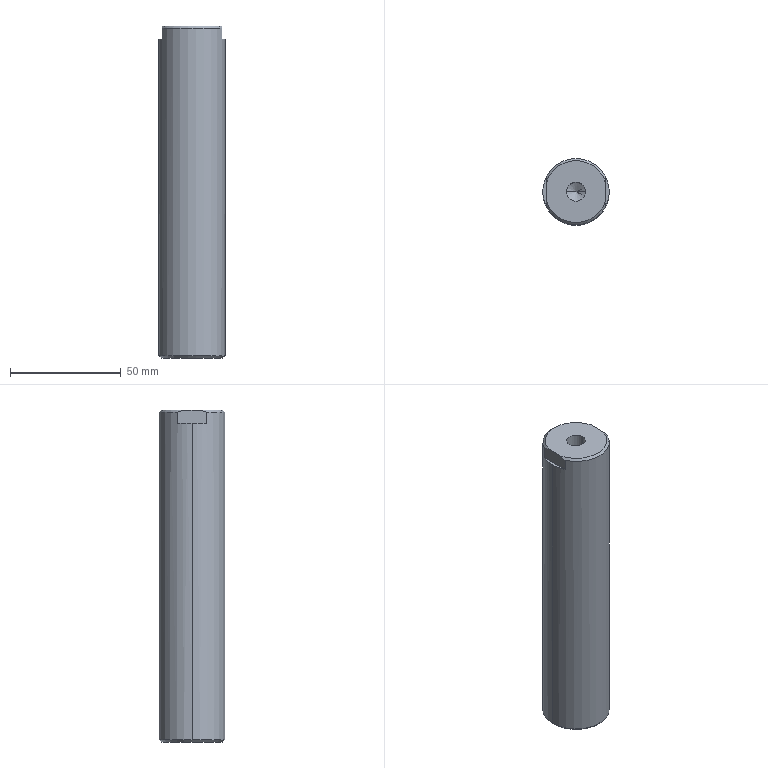Part | SolidWorks | features BaseBody 1 | 1 solid | 20 faces | box 30 x 30 x 150 mm | volume 102856 mm3 | cone 8 | cylinder 6 | plane 6 | commonest cylinder face diameters 8.5 x4 30 x2
STEP:
#1=CARTESIAN_POINT('',(-4.25,0.,125.));
#2=VERTEX_POINT('',#1);
#3=CARTESIAN_POINT('',(4.25,0.,125.));
#4=VERTEX_POINT('',#3);
#5=CARTESIAN_POINT('',(0.,0.,125.));
#6=DIRECTION('',(0.,0.,1.));
#7=DIRECTION('',(1.,0.,0.));
#8=AXIS2_PLACEMENT_3D('',#5,#6,#7);
#9=CIRCLE('',#8,4.25);
#10=EDGE_CURVE('',#2,#4,#9,.T.);
#11=ORIENTED_EDGE('',*,*,#10,.F.);
#12=CARTESIAN_POINT('',(-4.25,0.,150.));
#13=VERTEX_POINT('',#12);
#14=CARTESIAN_POINT('',(-4.25,0.,150.));
#15=DIRECTION('',(0.,0.,1.));
#16=VECTOR('',#15,1000.);
#17=LINE('',#14,#16);
#18=EDGE_CURVE('',#2,#13,#17,.T.);
#19=ORIENTED_EDGE('',*,*,#18,.T.);
#20=CARTESIAN_POINT('',(4.25,0.,150.));
#21=VERTEX_POINT('',#20);
#22=CARTESIAN_POINT('',(0.,0.,150.));
#23=DIRECTION('',(0.,0.,1.));
#24=DIRECTION('',(1.,0.,0.));
#25=AXIS2_PLACEMENT_3D('',#22,#23,#24);
#26=CIRCLE('',#25,4.25);
#27=EDGE_CURVE('',#13,#21,#26,.T.);
#28=ORIENTED_EDGE('',*,*,#27,.T.);
#29=CARTESIAN_POINT('',(4.25,0.,150.));
#30=DIRECTION('',(0.,0.,1.));
#31=VECTOR('',#30,1000.);
#32=LINE('',#29,#31);
#33=EDGE_CURVE('',#4,#21,#32,.T.);
#34=ORIENTED_EDGE('',*,*,#33,.F.);
#35=EDGE_LOOP('',(#11,#19,#28,#34));
#36=FACE_OUTER_BOUND('',#35,.T.);
#37=CARTESIAN_POINT('',(0.,0.,150.));
#38=DIRECTION('',(0.,0.,1.));
#39=DIRECTION('',(1.,0.,0.));
#40=AXIS2_PLACEMENT_3D('',#37,#38,#39);
#41=CYLINDRICAL_SURFACE('',#40,4.25);
#42=ADVANCED_FACE('',(#36),#41,.F.);
#43=CARTESIAN_POINT('',(0.,0.,122.446));
#44=VERTEX_POINT('',#43);
#45=CARTESIAN_POINT('',(4.25,0.,125.));
#46=DIRECTION('',(0.8572,0.,0.515));
#47=VECTOR('',#46,1000.);
#48=LINE('',#45,#47);
#49=EDGE_CURVE('',#44,#4,#48,.T.);
#50=ORIENTED_EDGE('',*,*,#49,.F.);
#51=CARTESIAN_POINT('',(-4.25,0.,125.));
#52=DIRECTION('',(-0.8572,0.,0.515));
#53=VECTOR('',#52,1000.);
#54=LINE('',#51,#53);
#55=EDGE_CURVE('',#44,#2,#54,.T.);
#56=ORIENTED_EDGE('',*,*,#55,.T.);
#57=ORIENTED_EDGE('',*,*,#10,.T.);
#58=EDGE_LOOP('',(#50,#56,#57));
#59=FACE_OUTER_BOUND('',#58,.T.);
#60=CARTESIAN_POINT('',(0.,0.,125.));
#61=DIRECTION('',(0.,0.,1.));
#62=DIRECTION('',(1.,0.,0.));
#63=AXIS2_PLACEMENT_3D('',#60,#61,#62);
#64=CONICAL_SURFACE('',#63,4.25,1.03);
#65=ADVANCED_FACE('',(#59),#64,.F.);
#66=CARTESIAN_POINT('',(4.25,0.,25.));
#67=VERTEX_POINT('',#66);
#68=CARTESIAN_POINT('',(-4.25,0.,25.));
#69=VERTEX_POINT('',#68);
#70=CARTESIAN_POINT('',(0.,0.,25.));
#71=DIRECTION('',(0.,0.,-1.));
#72=DIRECTION('',(-1.,0.,0.));
#73=AXIS2_PLACEMENT_3D('',#70,#71,#72);
#74=CIRCLE('',#73,4.25);
#75=EDGE_CURVE('',#67,#69,#74,.T.);
#76=ORIENTED_EDGE('',*,*,#75,.F.);
#77=CARTESIAN_POINT('',(4.25,0.,0.));
#78=VERTEX_POINT('',#77);
#79=CARTESIAN_POINT('',(4.25,0.,0.));
#80=DIRECTION('',(0.,0.,-1.));
#81=VECTOR('',#80,1000.);
#82=LINE('',#79,#81);
#83=EDGE_CURVE('',#67,#78,#82,.T.);
#84=ORIENTED_EDGE('',*,*,#83,.T.);
#85=CARTESIAN_POINT('',(-4.25,0.,0.));
#86=VERTEX_POINT('',#85);
#87=CARTESIAN_POINT('',(0.,0.,0.));
#88=DIRECTION('',(0.,0.,-1.));
#89=DIRECTION('',(-1.,0.,0.));
#90=AXIS2_PLACEMENT_3D('',#87,#88,#89);
#91=CIRCLE('',#90,4.25);
#92=EDGE_CURVE('',#78,#86,#91,.T.);
#93=ORIENTED_EDGE('',*,*,#92,.T.);
#94=CARTESIAN_POINT('',(-4.25,0.,0.));
#95=DIRECTION('',(0.,0.,-1.));
#96=VECTOR('',#95,1000.);
#97=LINE('',#94,#96);
#98=EDGE_CURVE('',#69,#86,#97,.T.);
#99=ORIENTED_EDGE('',*,*,#98,.F.);
#100=EDGE_LOOP('',(#76,#84,#93,#99));
#101=FACE_OUTER_BOUND('',#100,.T.);
#102=CARTESIAN_POINT('',(0.,0.,0.));
#103=DIRECTION('',(0.,0.,-1.));
#104=DIRECTION('',(-1.,0.,0.));
#105=AXIS2_PLACEMENT_3D('',#102,#103,#104);
#106=CYLINDRICAL_SURFACE('',#105,4.25);
#107=ADVANCED_FACE('',(#101),#106,.F.);
#108=CARTESIAN_POINT('',(0.,0.,27.554));
#109=VERTEX_POINT('',#108);
#110=CARTESIAN_POINT('',(-4.25,0.,25.));
#111=DIRECTION('',(-0.8572,0.,-0.515));
#112=VECTOR('',#111,1000.);
#113=LINE('',#110,#112);
#114=EDGE_CURVE('',#109,#69,#113,.T.);
#115=ORIENTED_EDGE('',*,*,#114,.F.);
#116=CARTESIAN_POINT('',(4.25,0.,25.));
#117=DIRECTION('',(0.8572,0.,-0.515));
#118=VECTOR('',#117,1000.);
#119=LINE('',#116,#118);
#120=EDGE_CURVE('',#109,#67,#119,.T.);
#121=ORIENTED_EDGE('',*,*,#120,.T.);
#122=ORIENTED_EDGE('',*,*,#75,.T.);
#123=EDGE_LOOP('',(#115,#121,#122));
#124=FACE_OUTER_BOUND('',#123,.T.);
#125=CARTESIAN_POINT('',(0.,0.,25.));
#126=DIRECTION('',(0.,0.,-1.));
#127=DIRECTION('',(-1.,0.,0.));
#128=AXIS2_PLACEMENT_3D('',#125,#126,#127);
#129=CONICAL_SURFACE('',#128,4.25,1.03);
#130=ADVANCED_FACE('',(#124),#129,.F.);
#131=CARTESIAN_POINT('',(-14.,0.,0.));
#132=VERTEX_POINT('',#131);
#133=CARTESIAN_POINT('',(14.,0.,0.));
#134=VERTEX_POINT('',#133);
#135=CARTESIAN_POINT('',(0.,0.,0.));
#136=DIRECTION('',(0.,0.,-1.));
#137=DIRECTION('',(1.,0.,0.));
#138=AXIS2_PLACEMENT_3D('',#135,#136,#137);
#139=CIRCLE('',#138,14.);
#140=EDGE_CURVE('',#132,#134,#139,.T.);
#141=ORIENTED_EDGE('',*,*,#140,.F.);
#142=CARTESIAN_POINT('',(-15.,0.,1.));
#143=VERTEX_POINT('',#142);
#144=CARTESIAN_POINT('',(-15.,0.,1.));
#145=DIRECTION('',(-0.7071,0.,0.7071));
#146=VECTOR('',#145,1000.);
#147=LINE('',#144,#146);
#148=EDGE_CURVE('',#132,#143,#147,.T.);
#149=ORIENTED_EDGE('',*,*,#148,.T.);
#150=CARTESIAN_POINT('',(15.,0.,1.));
#151=VERTEX_POINT('',#150);
#152=CARTESIAN_POINT('',(0.,0.,1.));
#153=DIRECTION('',(0.,0.,1.));
#154=DIRECTION('',(1.,0.,0.));
#155=AXIS2_PLACEMENT_3D('',#152,#153,#154);
#156=CIRCLE('',#155,15.);
#157=EDGE_CURVE('',#151,#143,#156,.T.);
#158=ORIENTED_EDGE('',*,*,#157,.F.);
#159=CARTESIAN_POINT('',(15.,0.,1.));
#160=DIRECTION('',(0.7071,0.,0.7071));
#161=VECTOR('',#160,1000.);
#162=LINE('',#159,#161);
#163=EDGE_CURVE('',#134,#151,#162,.T.);
#164=ORIENTED_EDGE('',*,*,#163,.F.);
#165=EDGE_LOOP('',(#141,#149,#158,#164));
#166=FACE_OUTER_BOUND('',#165,.T.);
#167=CARTESIAN_POINT('',(0.,0.,1.));
#168=DIRECTION('',(0.,0.,1.));
#169=DIRECTION('',(1.,0.,0.));
#170=AXIS2_PLACEMENT_3D('',#167,#168,#169);
#171=CONICAL_SURFACE('',#170,15.,0.7854);
#172=ADVANCED_FACE('',(#166),#171,.T.);
#173=CARTESIAN_POINT('',(15.,0.,144.));
#174=VERTEX_POINT('',#173);
#175=CARTESIAN_POINT('',(13.5,6.538,144.));
#176=VERTEX_POINT('',#175);
#177=CARTESIAN_POINT('',(0.,0.,144.));
#178=DIRECTION('',(0.,0.,1.));
#179=DIRECTION('',(1.,0.,0.));
#180=AXIS2_PLACEMENT_3D('',#177,#178,#179);
#181=CIRCLE('',#180,15.);
#182=EDGE_CURVE('',#174,#176,#181,.T.);
#183=ORIENTED_EDGE('',*,*,#182,.F.);
#184=CARTESIAN_POINT('',(15.,0.,150.));
#185=DIRECTION('',(0.,0.,-1.));
#186=VECTOR('',#185,1000.);
#187=LINE('',#184,#186);
#188=EDGE_CURVE('',#174,#151,#187,.T.);
#189=ORIENTED_EDGE('',*,*,#188,.T.);
#190=ORIENTED_EDGE('',*,*,#157,.T.);
#191=CARTESIAN_POINT('',(-15.,0.,144.));
#192=VERTEX_POINT('',#191);
#193=CARTESIAN_POINT('',(-15.,0.,150.));
#194=DIRECTION('',(0.,0.,-1.));
#195=VECTOR('',#194,1000.);
#196=LINE('',#193,#195);
#197=EDGE_CURVE('',#192,#143,#196,.T.);
#198=ORIENTED_EDGE('',*,*,#197,.F.);
#199=CARTESIAN_POINT('',(-13.5,6.538,144.));
#200=VERTEX_POINT('',#199);
#201=CARTESIAN_POINT('',(0.,0.,144.));
#202=DIRECTION('',(0.,0.,1.));
#203=DIRECTION('',(1.,0.,0.));
#204=AXIS2_PLACEMENT_3D('',#201,#202,#203);
#205=CIRCLE('',#204,15.);
#206=EDGE_CURVE('',#200,#192,#205,.T.);
#207=ORIENTED_EDGE('',*,*,#206,.F.);
#208=CARTESIAN_POINT('',(-13.5,6.538,149.));
#209=VERTEX_POINT('',#208);
#210=CARTESIAN_POINT('',(-13.5,6.538,150.));
#211=DIRECTION('',(0.,0.,1.));
#212=VECTOR('',#211,1000.);
#213=LINE('',#210,#212);
#214=EDGE_CURVE('',#200,#209,#213,.T.);
#215=ORIENTED_EDGE('',*,*,#214,.T.);
#216=CARTESIAN_POINT('',(13.5,6.538,149.));
#217=VERTEX_POINT('',#216);
#218=CARTESIAN_POINT('',(0.,0.,149.));
#219=DIRECTION('',(0.,0.,-1.));
#220=DIRECTION('',(1.,0.,0.));
#221=AXIS2_PLACEMENT_3D('',#218,#219,#220);
#222=CIRCLE('',#221,15.);
#223=EDGE_CURVE('',#209,#217,#222,.T.);
#224=ORIENTED_EDGE('',*,*,#223,.T.);
#225=CARTESIAN_POINT('',(13.5,6.538,150.));
#226=DIRECTION('',(0.,0.,-1.));
#227=VECTOR('',#226,1000.);
#228=LINE('',#225,#227);
#229=EDGE_CURVE('',#217,#176,#228,.T.);
#230=ORIENTED_EDGE('',*,*,#229,.T.);
#231=EDGE_LOOP('',(#183,#189,#190,#198,#207,#215,#224,#230));
#232=FACE_OUTER_BOUND('',#231,.T.);
#233=CARTESIAN_POINT('',(0.,0.,150.));
#234=DIRECTION('',(0.,0.,-1.));
#235=DIRECTION('',(-1.,0.,0.));
#236=AXIS2_PLACEMENT_3D('',#233,#234,#235);
#237=CYLINDRICAL_SURFACE('',#236,15.);
#238=ADVANCED_FACE('',(#232),#237,.T.);
#239=CARTESIAN_POINT('',(13.5,3.708,150.));
#240=VERTEX_POINT('',#239);
#241=CARTESIAN_POINT('',(13.5,6.538,149.));
#242=CARTESIAN_POINT('',(13.5,5.623,149.399));
#243=CARTESIAN_POINT('',(13.5,4.683,149.742));
#244=CARTESIAN_POINT('',(13.5,3.708,150.));
#245=B_SPLINE_CURVE_WITH_KNOTS('',3,(#241,#242,#243,#244),.UNSPECIFIED.,.F.,.F.,(4,4),(0.02935,0.03235),.UNSPECIFIED.);
#246=EDGE_CURVE('',#217,#240,#245,.T.);
#247=ORIENTED_EDGE('',*,*,#246,.F.);
#248=ORIENTED_EDGE('',*,*,#223,.F.);
#249=CARTESIAN_POINT('',(-13.5,3.708,150.));
#250=VERTEX_POINT('',#249);
#251=CARTESIAN_POINT('',(-13.5,3.708,150.));
#252=CARTESIAN_POINT('',(-13.5,4.19,149.872));
#253=CARTESIAN_POINT('',(-13.5,4.667,149.723));
#254=CARTESIAN_POINT('',(-13.5,5.612,149.387));
#255=CARTESIAN_POINT('',(-13.5,6.08,149.2));
#256=CARTESIAN_POINT('',(-13.5,6.538,149.));
#257=B_SPLINE_CURVE_WITH_KNOTS('',3,(#251,#252,#253,#254,#255,#256),.UNSPECIFIED.,.F.,.F.,(4,2,4),(0.03986,0.04136,0.04286),.UNSPECIFIED.);
#258=EDGE_CURVE('',#250,#209,#257,.T.);
#259=ORIENTED_EDGE('',*,*,#258,.F.);
#260=CARTESIAN_POINT('',(0.,0.,150.));
#261=DIRECTION('',(0.,0.,1.));
#262=DIRECTION('',(1.,0.,0.));
#263=AXIS2_PLACEMENT_3D('',#260,#261,#262);
#264=CIRCLE('',#263,14.);
#265=EDGE_CURVE('',#240,#250,#264,.T.);
#266=ORIENTED_EDGE('',*,*,#265,.F.);
#267=EDGE_LOOP('',(#247,#248,#259,#266));
#268=FACE_OUTER_BOUND('',#267,.T.);
#269=CARTESIAN_POINT('',(0.,0.,150.));
#270=DIRECTION('',(0.,0.,-1.));
#271=DIRECTION('',(-1.,0.,0.));
#272=AXIS2_PLACEMENT_3D('',#269,#270,#271);
#273=CONICAL_SURFACE('',#272,14.,0.7854);
#274=ADVANCED_FACE('',(#268),#273,.T.);
#275=ORIENTED_EDGE('',*,*,#188,.F.);
#276=CARTESIAN_POINT('',(13.5,-6.538,144.));
#277=VERTEX_POINT('',#276);
#278=CARTESIAN_POINT('',(0.,0.,144.));
#279=DIRECTION('',(0.,0.,1.));
#280=DIRECTION('',(1.,0.,0.));
#281=AXIS2_PLACEMENT_3D('',#278,#279,#280);
#282=CIRCLE('',#281,15.);
#283=EDGE_CURVE('',#277,#174,#282,.T.);
#284=ORIENTED_EDGE('',*,*,#283,.F.);
#285=CARTESIAN_POINT('',(13.5,-6.538,149.));
#286=VERTEX_POINT('',#285);
#287=CARTESIAN_POINT('',(13.5,-6.538,150.));
#288=DIRECTION('',(0.,0.,1.));
#289=VECTOR('',#288,1000.);
#290=LINE('',#287,#289);
#291=EDGE_CURVE('',#277,#286,#290,.T.);
#292=ORIENTED_EDGE('',*,*,#291,.T.);
#293=CARTESIAN_POINT('',(-13.5,-6.538,149.));
#294=VERTEX_POINT('',#293);
#295=CARTESIAN_POINT('',(0.,0.,149.));
#296=DIRECTION('',(0.,0.,-1.));
#297=DIRECTION('',(1.,0.,0.));
#298=AXIS2_PLACEMENT_3D('',#295,#296,#297);
#299=CIRCLE('',#298,15.);
#300=EDGE_CURVE('',#286,#294,#299,.T.);
#301=ORIENTED_EDGE('',*,*,#300,.T.);
#302=CARTESIAN_POINT('',(-13.5,-6.538,144.));
#303=VERTEX_POINT('',#302);
#304=CARTESIAN_POINT('',(-13.5,-6.538,150.));
#305=DIRECTION('',(0.,0.,-1.));
#306=VECTOR('',#305,1000.);
#307=LINE('',#304,#306);
#308=EDGE_CURVE('',#294,#303,#307,.T.);
#309=ORIENTED_EDGE('',*,*,#308,.T.);
#310=CARTESIAN_POINT('',(0.,0.,144.));
#311=DIRECTION('',(0.,0.,1.));
#312=DIRECTION('',(1.,0.,0.));
#313=AXIS2_PLACEMENT_3D('',#310,#311,#312);
#314=CIRCLE('',#313,15.);
#315=EDGE_CURVE('',#192,#303,#314,.T.);
#316=ORIENTED_EDGE('',*,*,#315,.F.);
#317=ORIENTED_EDGE('',*,*,#197,.T.);
#318=CARTESIAN_POINT('',(0.,0.,1.));
#319=DIRECTION('',(0.,0.,1.));
#320=DIRECTION('',(1.,0.,0.));
#321=AXIS2_PLACEMENT_3D('',#318,#319,#320);
#322=CIRCLE('',#321,15.);
#323=EDGE_CURVE('',#143,#151,#322,.T.);
#324=ORIENTED_EDGE('',*,*,#323,.T.);
#325=EDGE_LOOP('',(#275,#284,#292,#301,#309,#316,#317,#324));
#326=FACE_OUTER_BOUND('',#325,.T.);
#327=CARTESIAN_POINT('',(0.,0.,150.));
#328=DIRECTION('',(0.,0.,-1.));
#329=DIRECTION('',(-1.,0.,0.));
#330=AXIS2_PLACEMENT_3D('',#327,#328,#329);
#331=CYLINDRICAL_SURFACE('',#330,15.);
#332=ADVANCED_FACE('',(#326),#331,.T.);
#333=CARTESIAN_POINT('',(13.5,-3.708,150.));
#334=VERTEX_POINT('',#333);
#335=CARTESIAN_POINT('',(13.5,14.756,150.));
#336=DIRECTION('',(0.,-1.,0.));
#337=VECTOR('',#336,1000.);
#338=LINE('',#335,#337);
#339=EDGE_CURVE('',#240,#334,#338,.T.);
#340=ORIENTED_EDGE('',*,*,#339,.F.);
#341=ORIENTED_EDGE('',*,*,#265,.T.);
#342=CARTESIAN_POINT('',(-13.5,-3.708,150.));
#343=VERTEX_POINT('',#342);
#344=CARTESIAN_POINT('',(-13.5,14.756,150.));
#345=DIRECTION('',(0.,1.,0.));
#346=VECTOR('',#345,1000.);
#347=LINE('',#344,#346);
#348=EDGE_CURVE('',#343,#250,#347,.T.);
#349=ORIENTED_EDGE('',*,*,#348,.F.);
#350=CARTESIAN_POINT('',(0.,0.,150.));
#351=DIRECTION('',(0.,0.,1.));
#352=DIRECTION('',(1.,0.,0.));
#353=AXIS2_PLACEMENT_3D('',#350,#351,#352);
#354=CIRCLE('',#353,14.);
#355=EDGE_CURVE('',#343,#334,#354,.T.);
#356=ORIENTED_EDGE('',*,*,#355,.T.);
#357=EDGE_LOOP('',(#340,#341,#349,#356));
#358=FACE_OUTER_BOUND('',#357,.T.);
#359=CARTESIAN_POINT('',(0.,0.,150.));
#360=DIRECTION('',(0.,0.,1.));
#361=DIRECTION('',(1.,0.,0.));
#362=AXIS2_PLACEMENT_3D('',#359,#360,#361);
#363=CIRCLE('',#362,4.25);
#364=EDGE_CURVE('',#21,#13,#363,.T.);
#365=ORIENTED_EDGE('',*,*,#364,.F.);
#366=ORIENTED_EDGE('',*,*,#27,.F.);
#367=EDGE_LOOP('',(#365,#366));
#368=FACE_BOUND('',#367,.T.);
#369=CARTESIAN_POINT('',(0.,0.,150.));
#370=DIRECTION('',(0.,0.,1.));
#371=DIRECTION('',(1.,0.,0.));
#372=AXIS2_PLACEMENT_3D('',#369,#370,#371);
#373=PLANE('',#372);
#374=ADVANCED_FACE('',(#358,#368),#373,.T.);
#375=CARTESIAN_POINT('',(0.,0.,0.));
#376=DIRECTION('',(0.,0.,-1.));
#377=DIRECTION('',(-1.,0.,0.));
#378=AXIS2_PLACEMENT_3D('',#375,#376,#377);
#379=CIRCLE('',#378,4.25);
#380=EDGE_CURVE('',#86,#78,#379,.T.);
#381=ORIENTED_EDGE('',*,*,#380,.F.);
#382=ORIENTED_EDGE('',*,*,#92,.F.);
#383=EDGE_LOOP('',(#381,#382));
#384=FACE_BOUND('',#383,.T.);
#385=CARTESIAN_POINT('',(0.,0.,0.));
#386=DIRECTION('',(0.,0.,-1.));
#387=DIRECTION('',(1.,0.,0.));
#388=AXIS2_PLACEMENT_3D('',#385,#386,#387);
#389=CIRCLE('',#388,14.);
#390=EDGE_CURVE('',#134,#132,#389,.T.);
#391=ORIENTED_EDGE('',*,*,#390,.T.);
#392=ORIENTED_EDGE('',*,*,#140,.T.);
#393=EDGE_LOOP('',(#391,#392));
#394=FACE_OUTER_BOUND('',#393,.T.);
#395=CARTESIAN_POINT('',(0.,0.,0.));
#396=DIRECTION('',(0.,0.,1.));
#397=DIRECTION('',(1.,0.,0.));
#398=AXIS2_PLACEMENT_3D('',#395,#396,#397);
#399=PLANE('',#398);
#400=ADVANCED_FACE('',(#384,#394),#399,.F.);
#401=ORIENTED_EDGE('',*,*,#148,.F.);
#402=ORIENTED_EDGE('',*,*,#390,.F.);
#403=ORIENTED_EDGE('',*,*,#163,.T.);
#404=ORIENTED_EDGE('',*,*,#323,.F.);
#405=EDGE_LOOP('',(#401,#402,#403,#404));
#406=FACE_OUTER_BOUND('',#405,.T.);
#407=CARTESIAN_POINT('',(0.,0.,1.));
#408=DIRECTION('',(0.,0.,1.));
#409=DIRECTION('',(1.,0.,0.));
#410=AXIS2_PLACEMENT_3D('',#407,#408,#409);
#411=CONICAL_SURFACE('',#410,15.,0.7854);
#412=ADVANCED_FACE('',(#406),#411,.T.);
#413=CARTESIAN_POINT('',(13.5,-3.708,150.));
#414=CARTESIAN_POINT('',(13.5,-4.19,149.872));
#415=CARTESIAN_POINT('',(13.5,-4.667,149.723));
#416=CARTESIAN_POINT('',(13.5,-5.612,149.387));
#417=CARTESIAN_POINT('',(13.5,-6.08,149.2));
#418=CARTESIAN_POINT('',(13.5,-6.538,149.));
#419=B_SPLINE_CURVE_WITH_KNOTS('',3,(#413,#414,#415,#416,#417,#418),.UNSPECIFIED.,.F.,.F.,(4,2,4),(0.03986,0.04136,0.04286),.UNSPECIFIED.);
#420=EDGE_CURVE('',#334,#286,#419,.T.);
#421=ORIENTED_EDGE('',*,*,#420,.F.);
#422=ORIENTED_EDGE('',*,*,#355,.F.);
#423=CARTESIAN_POINT('',(-13.5,-6.538,149.));
#424=CARTESIAN_POINT('',(-13.5,-5.623,149.399));
#425=CARTESIAN_POINT('',(-13.5,-4.683,149.742));
#426=CARTESIAN_POINT('',(-13.5,-3.708,150.));
#427=B_SPLINE_CURVE_WITH_KNOTS('',3,(#423,#424,#425,#426),.UNSPECIFIED.,.F.,.F.,(4,4),(0.02935,0.03235),.UNSPECIFIED.);
#428=EDGE_CURVE('',#294,#343,#427,.T.);
#429=ORIENTED_EDGE('',*,*,#428,.F.);
#430=ORIENTED_EDGE('',*,*,#300,.F.);
#431=EDGE_LOOP('',(#421,#422,#429,#430));
#432=FACE_OUTER_BOUND('',#431,.T.);
#433=CARTESIAN_POINT('',(0.,0.,150.));
#434=DIRECTION('',(0.,0.,-1.));
#435=DIRECTION('',(-1.,0.,0.));
#436=AXIS2_PLACEMENT_3D('',#433,#434,#435);
#437=CONICAL_SURFACE('',#436,14.,0.7854);
#438=ADVANCED_FACE('',(#432),#437,.T.);
#439=ORIENTED_EDGE('',*,*,#120,.F.);
#440=ORIENTED_EDGE('',*,*,#114,.T.);
#441=CARTESIAN_POINT('',(0.,0.,25.));
#442=DIRECTION('',(0.,0.,-1.));
#443=DIRECTION('',(-1.,0.,0.));
#444=AXIS2_PLACEMENT_3D('',#441,#442,#443);
#445=CIRCLE('',#444,4.25);
#446=EDGE_CURVE('',#69,#67,#445,.T.);
#447=ORIENTED_EDGE('',*,*,#446,.T.);
#448=EDGE_LOOP('',(#439,#440,#447));
#449=FACE_OUTER_BOUND('',#448,.T.);
#450=CARTESIAN_POINT('',(0.,0.,25.));
#451=DIRECTION('',(0.,0.,-1.));
#452=DIRECTION('',(-1.,0.,0.));
#453=AXIS2_PLACEMENT_3D('',#450,#451,#452);
#454=CONICAL_SURFACE('',#453,4.25,1.03);
#455=ADVANCED_FACE('',(#449),#454,.F.);
#456=ORIENTED_EDGE('',*,*,#83,.F.);
#457=ORIENTED_EDGE('',*,*,#446,.F.);
#458=ORIENTED_EDGE('',*,*,#98,.T.);
#459=ORIENTED_EDGE('',*,*,#380,.T.);
#460=EDGE_LOOP('',(#456,#457,#458,#459));
#461=FACE_OUTER_BOUND('',#460,.T.);
#462=CARTESIAN_POINT('',(0.,0.,0.));
#463=DIRECTION('',(0.,0.,-1.));
#464=DIRECTION('',(-1.,0.,0.));
#465=AXIS2_PLACEMENT_3D('',#462,#463,#464);
#466=CYLINDRICAL_SURFACE('',#465,4.25);
#467=ADVANCED_FACE('',(#461),#466,.F.);
#468=ORIENTED_EDGE('',*,*,#55,.F.);
#469=ORIENTED_EDGE('',*,*,#49,.T.);
#470=CARTESIAN_POINT('',(0.,0.,125.));
#471=DIRECTION('',(0.,0.,1.));
#472=DIRECTION('',(1.,0.,0.));
#473=AXIS2_PLACEMENT_3D('',#470,#471,#472);
#474=CIRCLE('',#473,4.25);
#475=EDGE_CURVE('',#4,#2,#474,.T.);
#476=ORIENTED_EDGE('',*,*,#475,.T.);
#477=EDGE_LOOP('',(#468,#469,#476));
#478=FACE_OUTER_BOUND('',#477,.T.);
#479=CARTESIAN_POINT('',(0.,0.,125.));
#480=DIRECTION('',(0.,0.,1.));
#481=DIRECTION('',(1.,0.,0.));
#482=AXIS2_PLACEMENT_3D('',#479,#480,#481);
#483=CONICAL_SURFACE('',#482,4.25,1.03);
#484=ADVANCED_FACE('',(#478),#483,.F.);
#485=ORIENTED_EDGE('',*,*,#18,.F.);
#486=ORIENTED_EDGE('',*,*,#475,.F.);
#487=ORIENTED_EDGE('',*,*,#33,.T.);
#488=ORIENTED_EDGE('',*,*,#364,.T.);
#489=EDGE_LOOP('',(#485,#486,#487,#488));
#490=FACE_OUTER_BOUND('',#489,.T.);
#491=CARTESIAN_POINT('',(0.,0.,150.));
#492=DIRECTION('',(0.,0.,1.));
#493=DIRECTION('',(1.,0.,0.));
#494=AXIS2_PLACEMENT_3D('',#491,#492,#493);
#495=CYLINDRICAL_SURFACE('',#494,4.25);
#496=ADVANCED_FACE('',(#490),#495,.F.);
#497=ORIENTED_EDGE('',*,*,#206,.T.);
#498=ORIENTED_EDGE('',*,*,#315,.T.);
#499=CARTESIAN_POINT('',(-13.5,14.756,144.));
#500=DIRECTION('',(0.,1.,0.));
#501=VECTOR('',#500,1000.);
#502=LINE('',#499,#501);
#503=EDGE_CURVE('',#303,#200,#502,.T.);
#504=ORIENTED_EDGE('',*,*,#503,.T.);
#505=EDGE_LOOP('',(#497,#498,#504));
#506=FACE_OUTER_BOUND('',#505,.T.);
#507=CARTESIAN_POINT('',(0.,0.,144.));
#508=DIRECTION('',(0.,0.,1.));
#509=DIRECTION('',(1.,0.,0.));
#510=AXIS2_PLACEMENT_3D('',#507,#508,#509);
#511=PLANE('',#510);
#512=ADVANCED_FACE('',(#506),#511,.T.);
#513=ORIENTED_EDGE('',*,*,#428,.T.);
#514=ORIENTED_EDGE('',*,*,#348,.T.);
#515=ORIENTED_EDGE('',*,*,#258,.T.);
#516=ORIENTED_EDGE('',*,*,#214,.F.);
#517=ORIENTED_EDGE('',*,*,#503,.F.);
#518=ORIENTED_EDGE('',*,*,#308,.F.);
#519=EDGE_LOOP('',(#513,#514,#515,#516,#517,#518));
#520=FACE_OUTER_BOUND('',#519,.T.);
#521=CARTESIAN_POINT('',(-13.5,14.756,144.));
#522=DIRECTION('',(1.,0.,0.));
#523=DIRECTION('',(0.,0.,-1.));
#524=AXIS2_PLACEMENT_3D('',#521,#522,#523);
#525=PLANE('',#524);
#526=ADVANCED_FACE('',(#520),#525,.F.);
#527=ORIENTED_EDGE('',*,*,#283,.T.);
#528=ORIENTED_EDGE('',*,*,#182,.T.);
#529=CARTESIAN_POINT('',(13.5,14.756,144.));
#530=DIRECTION('',(0.,-1.,0.));
#531=VECTOR('',#530,1000.);
#532=LINE('',#529,#531);
#533=EDGE_CURVE('',#176,#277,#532,.T.);
#534=ORIENTED_EDGE('',*,*,#533,.T.);
#535=EDGE_LOOP('',(#527,#528,#534));
#536=FACE_OUTER_BOUND('',#535,.T.);
#537=CARTESIAN_POINT('',(0.,0.,144.));
#538=DIRECTION('',(0.,0.,1.));
#539=DIRECTION('',(1.,0.,0.));
#540=AXIS2_PLACEMENT_3D('',#537,#538,#539);
#541=PLANE('',#540);
#542=ADVANCED_FACE('',(#536),#541,.T.);
#543=ORIENTED_EDGE('',*,*,#246,.T.);
#544=ORIENTED_EDGE('',*,*,#339,.T.);
#545=ORIENTED_EDGE('',*,*,#420,.T.);
#546=ORIENTED_EDGE('',*,*,#291,.F.);
#547=ORIENTED_EDGE('',*,*,#533,.F.);
#548=ORIENTED_EDGE('',*,*,#229,.F.);
#549=EDGE_LOOP('',(#543,#544,#545,#546,#547,#548));
#550=FACE_OUTER_BOUND('',#549,.T.);
#551=CARTESIAN_POINT('',(13.5,14.756,144.));
#552=DIRECTION('',(-1.,0.,0.));
#553=DIRECTION('',(0.,0.,1.));
#554=AXIS2_PLACEMENT_3D('',#551,#552,#553);
#555=PLANE('',#554);
#556=ADVANCED_FACE('',(#550),#555,.F.);
#557=CLOSED_SHELL('',(#42,#65,#107,#130,#172,#238,#274,#332,#374,#400,#412,#438,#455,#467,#484,#496,#512,#526,#542,#556));
#558=MANIFOLD_SOLID_BREP('',#557);
#559=CARTESIAN_POINT('',(0.,0.,0.));
#560=DIRECTION('',(0.,0.,1.));
#561=DIRECTION('',(1.,0.,0.));
#562=AXIS2_PLACEMENT_3D('',#559,#560,#561);
#563=(LENGTH_UNIT()NAMED_UNIT(*)SI_UNIT(.MILLI.,.METRE.));
#564=UNCERTAINTY_MEASURE_WITH_UNIT(LENGTH_MEASURE(0.00001),#563,'','');
#565=(NAMED_UNIT(*)PLANE_ANGLE_UNIT()SI_UNIT($,.RADIAN.));
#566=(NAMED_UNIT(*)SI_UNIT($,.STERADIAN.)SOLID_ANGLE_UNIT());
#567=(GEOMETRIC_REPRESENTATION_CONTEXT(3)GLOBAL_UNCERTAINTY_ASSIGNED_CONTEXT((#564))GLOBAL_UNIT_ASSIGNED_CONTEXT((#563,#565,#566))REPRESENTATION_CONTEXT('',''));
#568=ADVANCED_BREP_SHAPE_REPRESENTATION('',(#558,#562),#567);